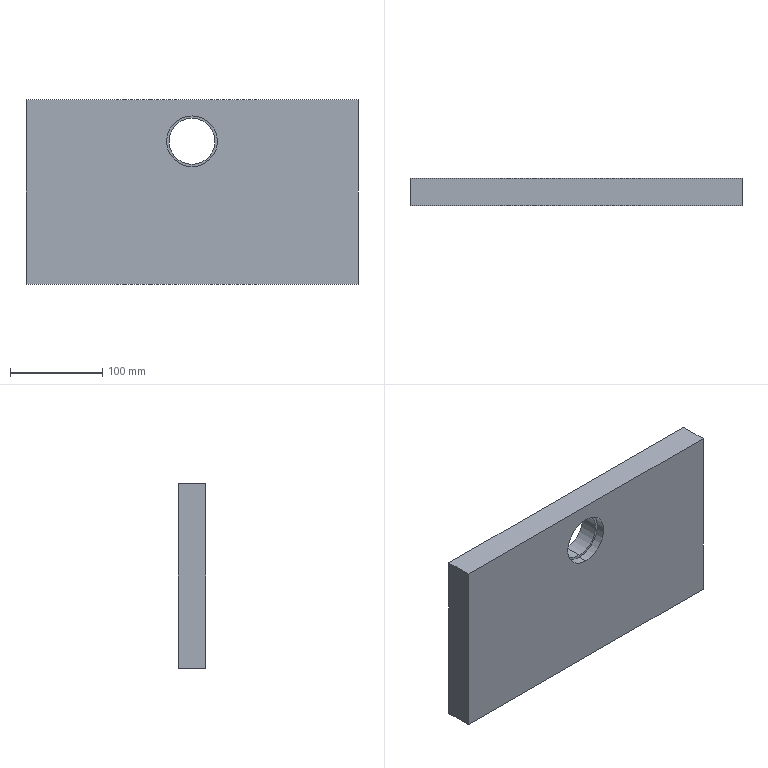Part | SolidWorks | features Cut 2, Extrusion 1 | 1 solid | 11 faces | box 360 x 30 x 200 mm | volume 2096972 mm3 | plane 7 | cylinder 4 | commonest cylinder face diameters 50 x2 55 x2
STEP:
#1=CARTESIAN_POINT('',(0.,10.,82.5));
#2=VERTEX_POINT('',#1);
#3=CARTESIAN_POINT('',(0.,10.,27.5));
#4=VERTEX_POINT('',#3);
#5=CARTESIAN_POINT('',(0.,10.,55.));
#6=DIRECTION('',(0.,-1.,0.));
#7=DIRECTION('',(0.,0.,-1.));
#8=AXIS2_PLACEMENT_3D('',#5,#6,#7);
#9=CIRCLE('',#8,27.5);
#10=EDGE_CURVE('',#2,#4,#9,.T.);
#11=ORIENTED_EDGE('',*,*,#10,.F.);
#12=CARTESIAN_POINT('',(0.,0.,82.5));
#13=VERTEX_POINT('',#12);
#14=CARTESIAN_POINT('',(0.,10.,82.5));
#15=DIRECTION('',(0.,-1.,0.));
#16=VECTOR('',#15,1000.);
#17=LINE('',#14,#16);
#18=EDGE_CURVE('',#2,#13,#17,.T.);
#19=ORIENTED_EDGE('',*,*,#18,.T.);
#20=CARTESIAN_POINT('',(0.,0.,27.5));
#21=VERTEX_POINT('',#20);
#22=CARTESIAN_POINT('',(0.,0.,55.));
#23=DIRECTION('',(0.,-1.,0.));
#24=DIRECTION('',(0.,0.,-1.));
#25=AXIS2_PLACEMENT_3D('',#22,#23,#24);
#26=CIRCLE('',#25,27.5);
#27=EDGE_CURVE('',#13,#21,#26,.T.);
#28=ORIENTED_EDGE('',*,*,#27,.T.);
#29=CARTESIAN_POINT('',(0.,10.,27.5));
#30=DIRECTION('',(0.,-1.,0.));
#31=VECTOR('',#30,1000.);
#32=LINE('',#29,#31);
#33=EDGE_CURVE('',#4,#21,#32,.T.);
#34=ORIENTED_EDGE('',*,*,#33,.F.);
#35=EDGE_LOOP('',(#11,#19,#28,#34));
#36=FACE_OUTER_BOUND('',#35,.T.);
#37=CARTESIAN_POINT('',(0.,10.,55.));
#38=DIRECTION('',(0.,-1.,0.));
#39=DIRECTION('',(0.,0.,-1.));
#40=AXIS2_PLACEMENT_3D('',#37,#38,#39);
#41=CYLINDRICAL_SURFACE('',#40,27.5);
#42=ADVANCED_FACE('',(#36),#41,.F.);
#43=CARTESIAN_POINT('',(0.,30.,80.));
#44=VERTEX_POINT('',#43);
#45=CARTESIAN_POINT('',(0.,30.,30.));
#46=VERTEX_POINT('',#45);
#47=CARTESIAN_POINT('',(0.,30.,55.));
#48=DIRECTION('',(0.,-1.,0.));
#49=DIRECTION('',(0.,0.,-1.));
#50=AXIS2_PLACEMENT_3D('',#47,#48,#49);
#51=CIRCLE('',#50,25.);
#52=EDGE_CURVE('',#44,#46,#51,.T.);
#53=ORIENTED_EDGE('',*,*,#52,.F.);
#54=CARTESIAN_POINT('',(0.,10.,80.));
#55=VERTEX_POINT('',#54);
#56=CARTESIAN_POINT('',(0.,30.,80.));
#57=DIRECTION('',(0.,-1.,0.));
#58=VECTOR('',#57,1000.);
#59=LINE('',#56,#58);
#60=EDGE_CURVE('',#44,#55,#59,.T.);
#61=ORIENTED_EDGE('',*,*,#60,.T.);
#62=CARTESIAN_POINT('',(0.,10.,30.));
#63=VERTEX_POINT('',#62);
#64=CARTESIAN_POINT('',(0.,10.,55.));
#65=DIRECTION('',(0.,1.,0.));
#66=DIRECTION('',(0.,0.,-1.));
#67=AXIS2_PLACEMENT_3D('',#64,#65,#66);
#68=CIRCLE('',#67,25.);
#69=EDGE_CURVE('',#63,#55,#68,.T.);
#70=ORIENTED_EDGE('',*,*,#69,.F.);
#71=CARTESIAN_POINT('',(0.,30.,30.));
#72=DIRECTION('',(0.,-1.,0.));
#73=VECTOR('',#72,1000.);
#74=LINE('',#71,#73);
#75=EDGE_CURVE('',#46,#63,#74,.T.);
#76=ORIENTED_EDGE('',*,*,#75,.F.);
#77=EDGE_LOOP('',(#53,#61,#70,#76));
#78=FACE_OUTER_BOUND('',#77,.T.);
#79=CARTESIAN_POINT('',(0.,30.,55.));
#80=DIRECTION('',(0.,-1.,0.));
#81=DIRECTION('',(0.,0.,-1.));
#82=AXIS2_PLACEMENT_3D('',#79,#80,#81);
#83=CYLINDRICAL_SURFACE('',#82,25.);
#84=ADVANCED_FACE('',(#78),#83,.F.);
#85=ORIENTED_EDGE('',*,*,#60,.F.);
#86=CARTESIAN_POINT('',(0.,30.,55.));
#87=DIRECTION('',(0.,-1.,0.));
#88=DIRECTION('',(0.,0.,-1.));
#89=AXIS2_PLACEMENT_3D('',#86,#87,#88);
#90=CIRCLE('',#89,25.);
#91=EDGE_CURVE('',#46,#44,#90,.T.);
#92=ORIENTED_EDGE('',*,*,#91,.F.);
#93=ORIENTED_EDGE('',*,*,#75,.T.);
#94=CARTESIAN_POINT('',(0.,10.,55.));
#95=DIRECTION('',(0.,1.,0.));
#96=DIRECTION('',(0.,0.,-1.));
#97=AXIS2_PLACEMENT_3D('',#94,#95,#96);
#98=CIRCLE('',#97,25.);
#99=EDGE_CURVE('',#55,#63,#98,.T.);
#100=ORIENTED_EDGE('',*,*,#99,.F.);
#101=EDGE_LOOP('',(#85,#92,#93,#100));
#102=FACE_OUTER_BOUND('',#101,.T.);
#103=CARTESIAN_POINT('',(0.,30.,55.));
#104=DIRECTION('',(0.,-1.,0.));
#105=DIRECTION('',(0.,0.,-1.));
#106=AXIS2_PLACEMENT_3D('',#103,#104,#105);
#107=CYLINDRICAL_SURFACE('',#106,25.);
#108=ADVANCED_FACE('',(#102),#107,.F.);
#109=CARTESIAN_POINT('',(180.,0.,100.));
#110=VERTEX_POINT('',#109);
#111=CARTESIAN_POINT('',(180.,0.,-100.));
#112=VERTEX_POINT('',#111);
#113=CARTESIAN_POINT('',(180.,0.,100.));
#114=DIRECTION('',(0.,0.,-1.));
#115=VECTOR('',#114,1000.);
#116=LINE('',#113,#115);
#117=EDGE_CURVE('',#110,#112,#116,.T.);
#118=ORIENTED_EDGE('',*,*,#117,.T.);
#119=CARTESIAN_POINT('',(180.,30.,-100.));
#120=VERTEX_POINT('',#119);
#121=CARTESIAN_POINT('',(180.,30.,-100.));
#122=DIRECTION('',(0.,-1.,0.));
#123=VECTOR('',#122,1000.);
#124=LINE('',#121,#123);
#125=EDGE_CURVE('',#120,#112,#124,.T.);
#126=ORIENTED_EDGE('',*,*,#125,.F.);
#127=CARTESIAN_POINT('',(180.,30.,100.));
#128=VERTEX_POINT('',#127);
#129=CARTESIAN_POINT('',(180.,30.,100.));
#130=DIRECTION('',(0.,0.,-1.));
#131=VECTOR('',#130,1000.);
#132=LINE('',#129,#131);
#133=EDGE_CURVE('',#128,#120,#132,.T.);
#134=ORIENTED_EDGE('',*,*,#133,.F.);
#135=CARTESIAN_POINT('',(180.,30.,100.));
#136=DIRECTION('',(0.,-1.,0.));
#137=VECTOR('',#136,1000.);
#138=LINE('',#135,#137);
#139=EDGE_CURVE('',#128,#110,#138,.T.);
#140=ORIENTED_EDGE('',*,*,#139,.T.);
#141=EDGE_LOOP('',(#118,#126,#134,#140));
#142=FACE_OUTER_BOUND('',#141,.T.);
#143=CARTESIAN_POINT('',(180.,30.,100.));
#144=DIRECTION('',(-1.,0.,0.));
#145=DIRECTION('',(0.,0.,1.));
#146=AXIS2_PLACEMENT_3D('',#143,#144,#145);
#147=PLANE('',#146);
#148=ADVANCED_FACE('',(#142),#147,.F.);
#149=CARTESIAN_POINT('',(-180.,0.,-100.));
#150=VERTEX_POINT('',#149);
#151=CARTESIAN_POINT('',(-180.,0.,-100.));
#152=DIRECTION('',(-1.,0.,0.));
#153=VECTOR('',#152,1000.);
#154=LINE('',#151,#153);
#155=EDGE_CURVE('',#112,#150,#154,.T.);
#156=ORIENTED_EDGE('',*,*,#155,.T.);
#157=CARTESIAN_POINT('',(-180.,30.,-100.));
#158=VERTEX_POINT('',#157);
#159=CARTESIAN_POINT('',(-180.,30.,-100.));
#160=DIRECTION('',(0.,-1.,0.));
#161=VECTOR('',#160,1000.);
#162=LINE('',#159,#161);
#163=EDGE_CURVE('',#158,#150,#162,.T.);
#164=ORIENTED_EDGE('',*,*,#163,.F.);
#165=CARTESIAN_POINT('',(-180.,30.,-100.));
#166=DIRECTION('',(-1.,0.,0.));
#167=VECTOR('',#166,1000.);
#168=LINE('',#165,#167);
#169=EDGE_CURVE('',#120,#158,#168,.T.);
#170=ORIENTED_EDGE('',*,*,#169,.F.);
#171=ORIENTED_EDGE('',*,*,#125,.T.);
#172=EDGE_LOOP('',(#156,#164,#170,#171));
#173=FACE_OUTER_BOUND('',#172,.T.);
#174=CARTESIAN_POINT('',(-180.,30.,-100.));
#175=DIRECTION('',(0.,0.,1.));
#176=DIRECTION('',(1.,0.,0.));
#177=AXIS2_PLACEMENT_3D('',#174,#175,#176);
#178=PLANE('',#177);
#179=ADVANCED_FACE('',(#173),#178,.F.);
#180=CARTESIAN_POINT('',(-180.,0.,100.));
#181=VERTEX_POINT('',#180);
#182=CARTESIAN_POINT('',(-180.,0.,100.));
#183=DIRECTION('',(0.,0.,1.));
#184=VECTOR('',#183,1000.);
#185=LINE('',#182,#184);
#186=EDGE_CURVE('',#150,#181,#185,.T.);
#187=ORIENTED_EDGE('',*,*,#186,.T.);
#188=CARTESIAN_POINT('',(-180.,30.,100.));
#189=VERTEX_POINT('',#188);
#190=CARTESIAN_POINT('',(-180.,30.,100.));
#191=DIRECTION('',(0.,-1.,0.));
#192=VECTOR('',#191,1000.);
#193=LINE('',#190,#192);
#194=EDGE_CURVE('',#189,#181,#193,.T.);
#195=ORIENTED_EDGE('',*,*,#194,.F.);
#196=CARTESIAN_POINT('',(-180.,30.,100.));
#197=DIRECTION('',(0.,0.,1.));
#198=VECTOR('',#197,1000.);
#199=LINE('',#196,#198);
#200=EDGE_CURVE('',#158,#189,#199,.T.);
#201=ORIENTED_EDGE('',*,*,#200,.F.);
#202=ORIENTED_EDGE('',*,*,#163,.T.);
#203=EDGE_LOOP('',(#187,#195,#201,#202));
#204=FACE_OUTER_BOUND('',#203,.T.);
#205=CARTESIAN_POINT('',(-180.,30.,100.));
#206=DIRECTION('',(1.,0.,0.));
#207=DIRECTION('',(0.,0.,-1.));
#208=AXIS2_PLACEMENT_3D('',#205,#206,#207);
#209=PLANE('',#208);
#210=ADVANCED_FACE('',(#204),#209,.F.);
#211=CARTESIAN_POINT('',(-180.,0.,100.));
#212=DIRECTION('',(1.,0.,0.));
#213=VECTOR('',#212,1000.);
#214=LINE('',#211,#213);
#215=EDGE_CURVE('',#181,#110,#214,.T.);
#216=ORIENTED_EDGE('',*,*,#215,.T.);
#217=ORIENTED_EDGE('',*,*,#139,.F.);
#218=CARTESIAN_POINT('',(-180.,30.,100.));
#219=DIRECTION('',(1.,0.,0.));
#220=VECTOR('',#219,1000.);
#221=LINE('',#218,#220);
#222=EDGE_CURVE('',#189,#128,#221,.T.);
#223=ORIENTED_EDGE('',*,*,#222,.F.);
#224=ORIENTED_EDGE('',*,*,#194,.T.);
#225=EDGE_LOOP('',(#216,#217,#223,#224));
#226=FACE_OUTER_BOUND('',#225,.T.);
#227=CARTESIAN_POINT('',(-180.,30.,100.));
#228=DIRECTION('',(0.,0.,-1.));
#229=DIRECTION('',(-1.,0.,0.));
#230=AXIS2_PLACEMENT_3D('',#227,#228,#229);
#231=PLANE('',#230);
#232=ADVANCED_FACE('',(#226),#231,.F.);
#233=ORIENTED_EDGE('',*,*,#91,.T.);
#234=ORIENTED_EDGE('',*,*,#52,.T.);
#235=EDGE_LOOP('',(#233,#234));
#236=FACE_BOUND('',#235,.T.);
#237=ORIENTED_EDGE('',*,*,#133,.T.);
#238=ORIENTED_EDGE('',*,*,#169,.T.);
#239=ORIENTED_EDGE('',*,*,#200,.T.);
#240=ORIENTED_EDGE('',*,*,#222,.T.);
#241=EDGE_LOOP('',(#237,#238,#239,#240));
#242=FACE_OUTER_BOUND('',#241,.T.);
#243=CARTESIAN_POINT('',(0.,30.,0.));
#244=DIRECTION('',(0.,-1.,0.));
#245=DIRECTION('',(0.,0.,-1.));
#246=AXIS2_PLACEMENT_3D('',#243,#244,#245);
#247=PLANE('',#246);
#248=ADVANCED_FACE('',(#236,#242),#247,.F.);
#249=CARTESIAN_POINT('',(0.,0.,55.));
#250=DIRECTION('',(0.,-1.,0.));
#251=DIRECTION('',(0.,0.,-1.));
#252=AXIS2_PLACEMENT_3D('',#249,#250,#251);
#253=CIRCLE('',#252,27.5);
#254=EDGE_CURVE('',#21,#13,#253,.T.);
#255=ORIENTED_EDGE('',*,*,#254,.F.);
#256=ORIENTED_EDGE('',*,*,#27,.F.);
#257=EDGE_LOOP('',(#255,#256));
#258=FACE_BOUND('',#257,.T.);
#259=ORIENTED_EDGE('',*,*,#117,.F.);
#260=ORIENTED_EDGE('',*,*,#215,.F.);
#261=ORIENTED_EDGE('',*,*,#186,.F.);
#262=ORIENTED_EDGE('',*,*,#155,.F.);
#263=EDGE_LOOP('',(#259,#260,#261,#262));
#264=FACE_OUTER_BOUND('',#263,.T.);
#265=CARTESIAN_POINT('',(0.,0.,0.));
#266=DIRECTION('',(0.,-1.,0.));
#267=DIRECTION('',(0.,0.,-1.));
#268=AXIS2_PLACEMENT_3D('',#265,#266,#267);
#269=PLANE('',#268);
#270=ADVANCED_FACE('',(#258,#264),#269,.T.);
#271=CARTESIAN_POINT('',(0.,10.,55.));
#272=DIRECTION('',(0.,-1.,0.));
#273=DIRECTION('',(0.,0.,-1.));
#274=AXIS2_PLACEMENT_3D('',#271,#272,#273);
#275=CIRCLE('',#274,27.5);
#276=EDGE_CURVE('',#4,#2,#275,.T.);
#277=ORIENTED_EDGE('',*,*,#276,.T.);
#278=ORIENTED_EDGE('',*,*,#10,.T.);
#279=EDGE_LOOP('',(#277,#278));
#280=FACE_OUTER_BOUND('',#279,.T.);
#281=ORIENTED_EDGE('',*,*,#69,.T.);
#282=ORIENTED_EDGE('',*,*,#99,.T.);
#283=EDGE_LOOP('',(#281,#282));
#284=FACE_BOUND('',#283,.T.);
#285=CARTESIAN_POINT('',(0.,10.,55.));
#286=DIRECTION('',(0.,-1.,0.));
#287=DIRECTION('',(0.,0.,-1.));
#288=AXIS2_PLACEMENT_3D('',#285,#286,#287);
#289=PLANE('',#288);
#290=ADVANCED_FACE('',(#280,#284),#289,.T.);
#291=ORIENTED_EDGE('',*,*,#18,.F.);
#292=ORIENTED_EDGE('',*,*,#276,.F.);
#293=ORIENTED_EDGE('',*,*,#33,.T.);
#294=ORIENTED_EDGE('',*,*,#254,.T.);
#295=EDGE_LOOP('',(#291,#292,#293,#294));
#296=FACE_OUTER_BOUND('',#295,.T.);
#297=CARTESIAN_POINT('',(0.,10.,55.));
#298=DIRECTION('',(0.,-1.,0.));
#299=DIRECTION('',(0.,0.,-1.));
#300=AXIS2_PLACEMENT_3D('',#297,#298,#299);
#301=CYLINDRICAL_SURFACE('',#300,27.5);
#302=ADVANCED_FACE('',(#296),#301,.F.);
#303=CLOSED_SHELL('',(#42,#84,#108,#148,#179,#210,#232,#248,#270,#290,#302));
#304=MANIFOLD_SOLID_BREP('',#303);
#305=CARTESIAN_POINT('',(0.,0.,0.));
#306=DIRECTION('',(0.,0.,1.));
#307=DIRECTION('',(1.,0.,0.));
#308=AXIS2_PLACEMENT_3D('',#305,#306,#307);
#309=(LENGTH_UNIT()NAMED_UNIT(*)SI_UNIT(.MILLI.,.METRE.));
#310=UNCERTAINTY_MEASURE_WITH_UNIT(LENGTH_MEASURE(0.00001),#309,'','');
#311=(NAMED_UNIT(*)PLANE_ANGLE_UNIT()SI_UNIT($,.RADIAN.));
#312=(NAMED_UNIT(*)SI_UNIT($,.STERADIAN.)SOLID_ANGLE_UNIT());
#313=(GEOMETRIC_REPRESENTATION_CONTEXT(3)GLOBAL_UNCERTAINTY_ASSIGNED_CONTEXT((#310))GLOBAL_UNIT_ASSIGNED_CONTEXT((#309,#311,#312))REPRESENTATION_CONTEXT('',''));
#314=ADVANCED_BREP_SHAPE_REPRESENTATION('',(#304,#308),#313);